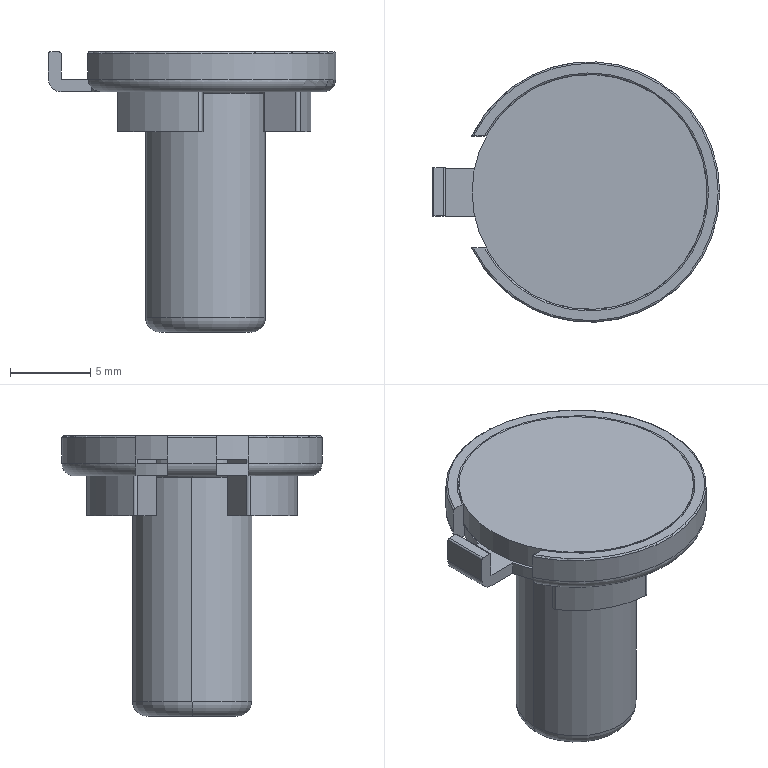NC program | NX | posted with a generic post | part box 17.958 x 16.273 x 17.5 mm
Whole program:
N10 G17 G21 G94 G90
(DRILLING , TOOL : ZXZ)
N12 T01 M6
N14 G54
N16 G17 G0 G90 X1.379 Y1.379 S5000 M3
N18 G43 Z30. H1
N20 G94 G81 G98 Z-0.55 F250. R3.
N22 X0. Y1.95
N24 X-1.379 Y1.379
N26 X-1.95 Y0.
N28 X-1.379 Y-1.379
N30 X0. Y-1.95
N32 X1.379 Y-1.379
N34 X1.95 Y0.
N36 G80
N38 G0 X1.95 Y0. Z30.
N40 M5
(DRILLING_COPY , TOOL : 1.0ZT)
N42 T11 M6
N44 G54
N46 G17 G0 G90 X1.379 Y1.379 S2000 M3
N48 G43 Z30. H11
N50 G94 G83 G98 Z-2.6 F100. Q1. R3.
N52 X0. Y1.95
N54 X-1.379 Y1.379
N56 X-1.95 Y0.
N58 X-1.379 Y-1.379
N60 X0. Y-1.95
N62 X1.379 Y-1.379
N64 X1.95 Y0.
N66 G80
N68 G0 X1.95 Y0. Z30.
N70 M5
(ZLEVEL_PROFILE_1 , TOOL : D4R0.5)
N72 T05 M6
N74 G54
N76 G17 G0 G90 X8.81 Y-4.672 S7500 M3
N78 G43 Z30. H5
N80 Z-14.01
N82 G94 G1 Z-15.01 F1000.
N84 X8.464 Y-4.072
N86 G3 X8.117 Y-3.872 R0.4
N88 G1 X7.937 Y-4.235 F2500.
N90 G2 X7.937 Y4.235 R-8.997
N92 G1 X7.967 Y4.097
N94 X8.089 Y3.872
N96 X8.211 Y3.879 Z-15.024
N98 X8.03 Y4.245
N100 G3 X8.03 Y-4.246 R-9.083
N102 G1 X8.061 Y-4.097
N104 X8.179 Y-3.879
N106 X8.295 Y-3.889 Z-15.042
N108 X8.116 Y-4.255
N110 G2 X8.116 Y4.255 R-9.164
N112 G1 X8.296 Y3.889
N114 X8.38 Y3.901 Z-15.065
N116 X8.276 Y4.097
N118 X8.201 Y4.264
N120 G3 X8.201 Y-4.264 R-9.243
N122 G1 X8.387 Y-3.901
N124 X8.461 Y-3.914 Z-15.093
N126 X8.368 Y-4.097
N128 X8.284 Y-4.273
N130 G2 X8.284 Y4.273 R-9.321
N132 G1 X8.467 Y3.914
N134 X8.54 Y3.928 Z-15.126
N136 X8.363 Y4.282
N138 G3 X8.363 Y-4.282 R-9.396
N140 G1 X8.539 Y-3.928
N142 X8.612 Y-3.942 Z-15.163
N144 X8.481 Y-4.202
N146 X8.44 Y-4.29
N148 G2 X8.44 Y4.29 R-9.468
N150 G1 X8.616 Y3.942
N152 X8.683 Y3.955 Z-15.205
N154 X8.514 Y4.297
N156 G3 X8.514 Y-4.297 R-9.537
N158 G1 X8.684 Y-3.955
N160 X8.751 Y-3.968 Z-15.251
N162 X8.585 Y-4.305
N164 G2 X8.585 Y4.305 R-9.604
N166 G1 X8.753 Y3.968
N168 X8.817 Y3.98 Z-15.3
N170 X8.653 Y4.312
N172 G3 X8.653 Y-4.311 R-9.668
N174 G1 X8.817 Y-3.98
N176 X8.876 Y-3.989 Z-15.353
N178 X8.717 Y-4.318
N180 G2 X8.717 Y4.318 R-9.728
N182 G1 X8.762 Y4.219
N184 X8.875 Y3.989
N186 X8.937 Y3.996 Z-15.41
N188 X8.777 Y4.324
N190 G3 X8.777 Y-4.324 R-9.785
N192 G1 X8.937 Y-3.996
N194 X8.995 Y-3.998 Z-15.471
N196 X8.834 Y-4.33
N198 G2 X8.834 Y4.33 R-9.838
N200 G1 X8.996 Y3.997
N202 X9.042 Y4. Z-15.534
N204 X9.021 Y4.047
N206 G3 X9.029 Y-4.028 R-9.887
N208 G1 X9.042 Y-4.
N210 X9.098 Z-15.6
N212 X8.934 Y-4.34
N214 G2 X8.934 Y4.34 R-9.932
N216 G1 X9.098 Y4.
N218 X9.139 Z-15.669
N220 X9.043 Y4.203
N222 X8.978 Y4.344
N224 G3 X8.978 Y-4.344 R-9.973
N226 G1 X9.141 Y-4.
N228 X9.181 Z-15.74
N230 X9.043 Y-4.289
N232 X9.017 Y-4.347
N234 G2 X9.017 Y4.348 R-10.01
N236 G1 X9.181 Y4.
N238 X9.218 Z-15.814
N240 X9.051 Y4.351
N242 G3 X9.051 Y-4.351 R-10.042
N244 G1 X9.218 Y-4.
N246 X9.248 Z-15.889
N248 X9.08 Y-4.354
N250 G2 X9.08 Y4.354 R-10.07
N252 G1 X9.247 Y4.
N254 X9.273 Z-15.966
N256 X9.104 Y4.356
N258 G3 X9.104 Y-4.356 R-10.093
N260 G1 X9.273 Y-4.
N262 X9.294 Z-16.044
N264 X9.124 Y-4.358
N266 G2 X9.124 Y4.358 R-10.111
N268 G1 X9.294 Y4.
N270 X9.304 Z-16.108
N272 X9.136 Y4.359
N274 G3 X9.211 Y-4.198 R-10.122
N276 G2 X9.302 Y-4. R29.49
N278 G1 X9.313 Z-16.172
N280 X9.144 Y-4.36
N282 G2 X9.144 Y4.36 R-10.13
N284 G1 X9.313 Y4.
N286 X9.319 Z-16.236
N288 X9.149 Y4.361
N290 G3 X9.149 Y-4.361 R-10.135
N292 G1 X9.32 Y-4.
N294 X9.321 Z-16.3
N296 X9.141 Y-4.379
N298 G2 X8.201 Y-5.956 R10.12
N300 X7.359 Y-6.969 R8.985
N302 G1 X7.261 Y-7.069
N304 X7.262 Y-7.07
N306 X6.709 Y-7.616
N308 G2 X5.676 Y-8.4 R17.985
N310 G1 X5.673 Y-8.397
N312 X5.059 Y-8.791
N314 X4.345 Y-9.158
N316 G2 X1.501 Y-10.028 R10.465
N318 X-1.169 Y-10.068 R10.169
N320 X-2.561 Y-9.804 R10.101
N322 G1 X-3.115 Y-9.652
N324 G2 X-4.155 Y-9.244 R13.078
N326 X-5.279 Y-8.652 R9.605
N328 G1 X-5.448 Y-8.546
N330 G2 X-7.657 Y-6.64 R10.208
N332 G1 X-8.021 Y-6.211
N334 X-8.367 Y-5.721
N336 X-8.437 Y-5.615
N338 G2 X-9.97 Y-1.861 R10.288
N340 G1 X-10.052 Y-1.305
N342 X-10.097 Y-0.833
N344 G2 X-10.101 Y0.76 R8.639
N346 X-9.545 Y3.396 R9.564
N348 X-8.767 Y5.113 R10.985
N350 G1 X-8.317 Y5.792
N352 X-7.977 Y6.275
N354 X-7.177 Y7.177
N356 X-6.596 Y7.696
N358 X-6.351 Y7.9
N360 G2 X0.619 Y10.116 R10.141
N362 X9.141 Y4.379 R10.135
N364 G1 X9.321 Y4.
N366 G3 X9.667 Y4.2 R0.4
N368 G1 X10.011 Y4.795
N370 Z-15.3
N372 G0 Z30.
N374 M5
N376 M2